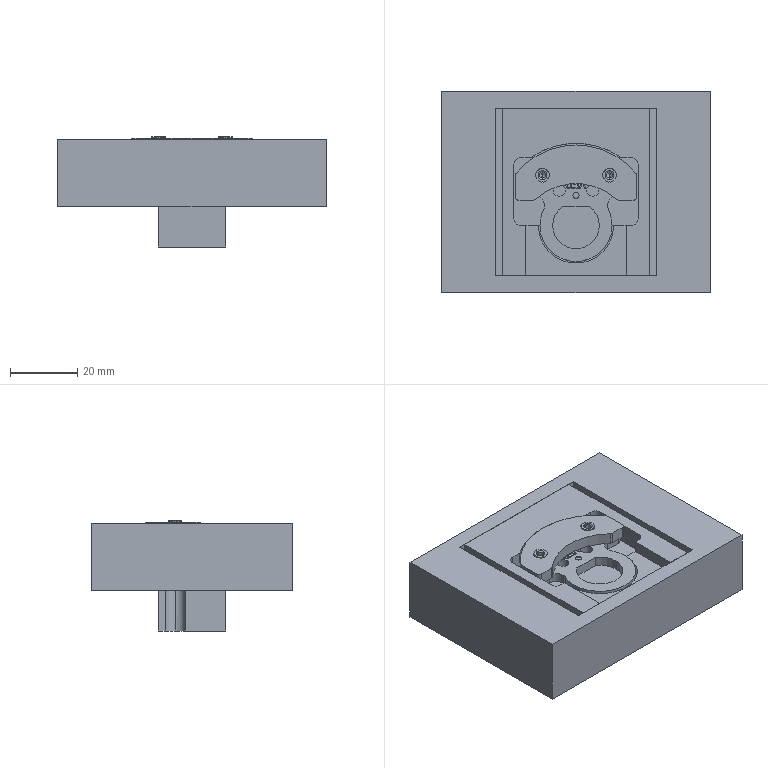Part | SolidWorks | features InContextFeatHolder 6 | 6 solids | 185 faces | box 80 x 60 x 32.8 mm | volume 73982 mm3 | plane 88 | cylinder 65 | cone 24 | spline 4 | torus 4 | commonest cylinder face diameters 4 x14 2 x12 3.2 x8 6 x7 3 x4 3.6 x4